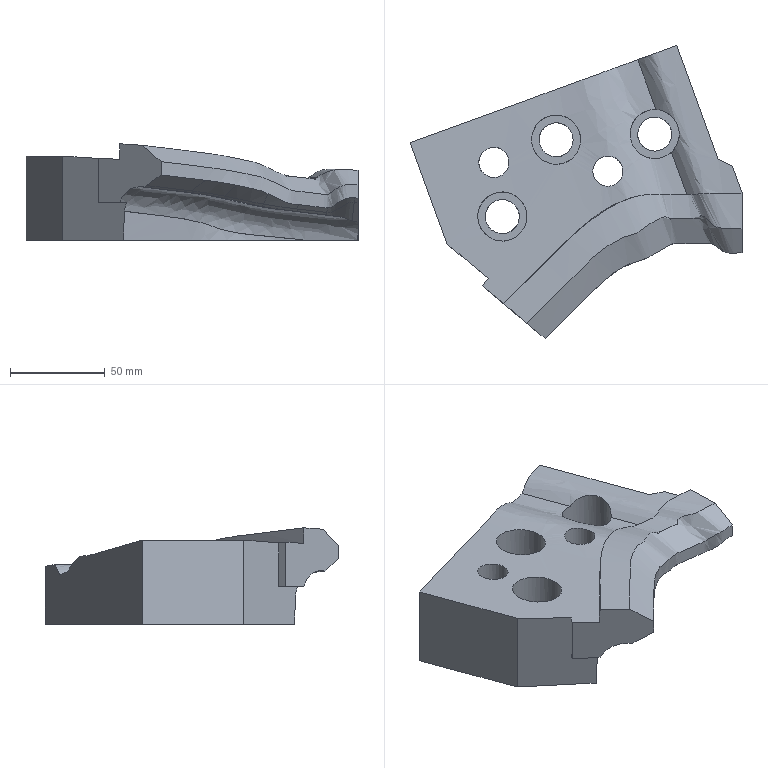Part | NX | features solid 2 | 1 solid | 51 faces | box 175.451 x 154.869 x 50.973 mm | volume 438476 mm3 | spline 29 | plane 14 | cylinder 8 | commonest cylinder face diameters 18 x3 26 x3 16 x2